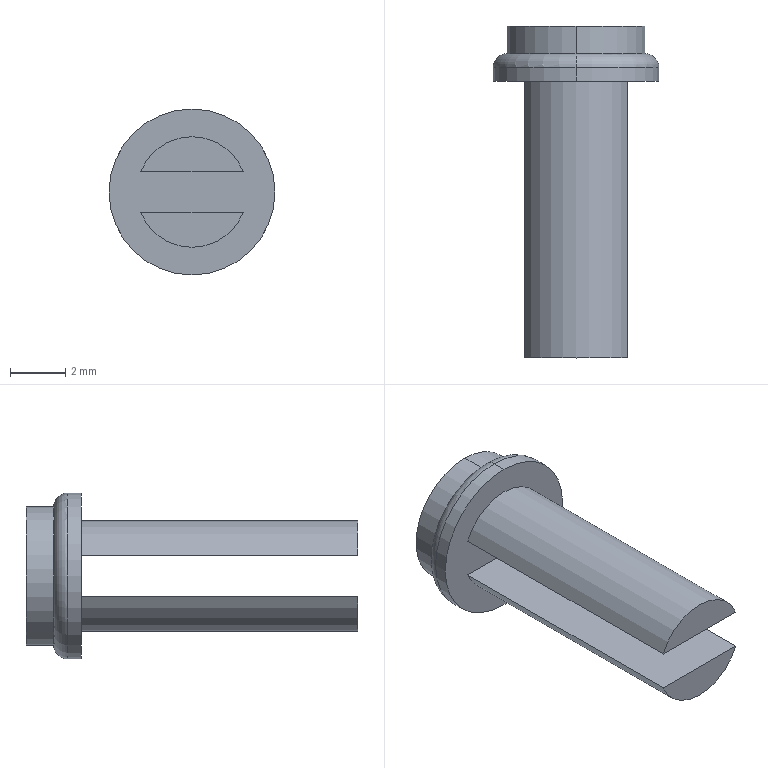Part | SolidWorks | features ICE 4, Extrusion 1, Fillet 1 | 1 solid | 28 faces | box 6 x 12 x 6 mm | volume 108.459 mm3 | plane 19 | cylinder 7 | torus 2 | commonest cylinder face diameters 4 x3 5 x2 6 x2
STEP:
#1=CARTESIAN_POINT('',(0.,10.5,-3.));
#2=VERTEX_POINT('',#1);
#3=CARTESIAN_POINT('',(0.,10.5,3.));
#4=VERTEX_POINT('',#3);
#5=CARTESIAN_POINT('',(0.,10.5,0.));
#6=DIRECTION('',(0.,-1.,0.));
#7=DIRECTION('',(0.,0.,1.));
#8=AXIS2_PLACEMENT_3D('',#5,#6,#7);
#9=CIRCLE('',#8,3.);
#10=EDGE_CURVE('',#2,#4,#9,.T.);
#11=ORIENTED_EDGE('',*,*,#10,.F.);
#12=CARTESIAN_POINT('',(0.,11.,-2.5));
#13=VERTEX_POINT('',#12);
#14=CARTESIAN_POINT('',(0.,10.5,-2.5));
#15=DIRECTION('',(1.,0.,0.));
#16=DIRECTION('',(0.,0.,-1.));
#17=AXIS2_PLACEMENT_3D('',#14,#15,#16);
#18=CIRCLE('',#17,0.5);
#19=EDGE_CURVE('',#2,#13,#18,.T.);
#20=ORIENTED_EDGE('',*,*,#19,.T.);
#21=CARTESIAN_POINT('',(0.,11.,2.5));
#22=VERTEX_POINT('',#21);
#23=CARTESIAN_POINT('',(0.,11.,0.));
#24=DIRECTION('',(0.,1.,0.));
#25=DIRECTION('',(0.,0.,1.));
#26=AXIS2_PLACEMENT_3D('',#23,#24,#25);
#27=CIRCLE('',#26,2.5);
#28=EDGE_CURVE('',#22,#13,#27,.T.);
#29=ORIENTED_EDGE('',*,*,#28,.F.);
#30=CARTESIAN_POINT('',(0.,10.5,2.5));
#31=DIRECTION('',(-1.,0.,0.));
#32=DIRECTION('',(0.,0.,1.));
#33=AXIS2_PLACEMENT_3D('',#30,#31,#32);
#34=CIRCLE('',#33,0.5);
#35=EDGE_CURVE('',#4,#22,#34,.T.);
#36=ORIENTED_EDGE('',*,*,#35,.F.);
#37=EDGE_LOOP('',(#11,#20,#29,#36));
#38=FACE_OUTER_BOUND('',#37,.T.);
#39=CARTESIAN_POINT('',(0.,10.5,0.));
#40=DIRECTION('',(0.,1.,0.));
#41=DIRECTION('',(0.,0.,1.));
#42=AXIS2_PLACEMENT_3D('',#39,#40,#41);
#43=TOROIDAL_SURFACE('',#42,2.5,0.5);
#44=ADVANCED_FACE('',(#38),#43,.T.);
#45=CARTESIAN_POINT('',(0.,12.,2.5));
#46=VERTEX_POINT('',#45);
#47=CARTESIAN_POINT('',(0.,12.,-2.5));
#48=VERTEX_POINT('',#47);
#49=CARTESIAN_POINT('',(0.,12.,0.));
#50=DIRECTION('',(0.,1.,0.));
#51=DIRECTION('',(0.,0.,1.));
#52=AXIS2_PLACEMENT_3D('',#49,#50,#51);
#53=CIRCLE('',#52,2.5);
#54=EDGE_CURVE('',#46,#48,#53,.T.);
#55=ORIENTED_EDGE('',*,*,#54,.F.);
#56=CARTESIAN_POINT('',(0.,12.,2.5));
#57=DIRECTION('',(0.,-1.,0.));
#58=VECTOR('',#57,1000.);
#59=LINE('',#56,#58);
#60=EDGE_CURVE('',#46,#22,#59,.T.);
#61=ORIENTED_EDGE('',*,*,#60,.T.);
#62=ORIENTED_EDGE('',*,*,#28,.T.);
#63=CARTESIAN_POINT('',(0.,12.,-2.5));
#64=DIRECTION('',(0.,-1.,0.));
#65=VECTOR('',#64,1000.);
#66=LINE('',#63,#65);
#67=EDGE_CURVE('',#48,#13,#66,.T.);
#68=ORIENTED_EDGE('',*,*,#67,.F.);
#69=EDGE_LOOP('',(#55,#61,#62,#68));
#70=FACE_OUTER_BOUND('',#69,.T.);
#71=CARTESIAN_POINT('',(0.,12.,0.));
#72=DIRECTION('',(0.,-1.,0.));
#73=DIRECTION('',(0.,0.,-1.));
#74=AXIS2_PLACEMENT_3D('',#71,#72,#73);
#75=CYLINDRICAL_SURFACE('',#74,2.5);
#76=ADVANCED_FACE('',(#70),#75,.T.);
#77=ORIENTED_EDGE('',*,*,#10,.T.);
#78=CARTESIAN_POINT('',(0.,10.,3.));
#79=VERTEX_POINT('',#78);
#80=CARTESIAN_POINT('',(0.,11.,3.));
#81=DIRECTION('',(0.,-1.,0.));
#82=VECTOR('',#81,1000.);
#83=LINE('',#80,#82);
#84=EDGE_CURVE('',#4,#79,#83,.T.);
#85=ORIENTED_EDGE('',*,*,#84,.T.);
#86=CARTESIAN_POINT('',(0.,10.,-3.));
#87=VERTEX_POINT('',#86);
#88=CARTESIAN_POINT('',(0.,10.,0.));
#89=DIRECTION('',(0.,1.,0.));
#90=DIRECTION('',(0.,0.,1.));
#91=AXIS2_PLACEMENT_3D('',#88,#89,#90);
#92=CIRCLE('',#91,3.);
#93=EDGE_CURVE('',#79,#87,#92,.T.);
#94=ORIENTED_EDGE('',*,*,#93,.T.);
#95=CARTESIAN_POINT('',(0.,11.,-3.));
#96=DIRECTION('',(0.,-1.,0.));
#97=VECTOR('',#96,1000.);
#98=LINE('',#95,#97);
#99=EDGE_CURVE('',#2,#87,#98,.T.);
#100=ORIENTED_EDGE('',*,*,#99,.F.);
#101=EDGE_LOOP('',(#77,#85,#94,#100));
#102=FACE_OUTER_BOUND('',#101,.T.);
#103=CARTESIAN_POINT('',(0.,11.,0.));
#104=DIRECTION('',(0.,-1.,0.));
#105=DIRECTION('',(0.,0.,-1.));
#106=AXIS2_PLACEMENT_3D('',#103,#104,#105);
#107=CYLINDRICAL_SURFACE('',#106,3.);
#108=ADVANCED_FACE('',(#102),#107,.T.);
#109=CARTESIAN_POINT('',(0.,10.,-2.));
#110=VERTEX_POINT('',#109);
#111=CARTESIAN_POINT('',(-1.854,10.,-0.75));
#112=VERTEX_POINT('',#111);
#113=CARTESIAN_POINT('',(0.,10.,0.));
#114=DIRECTION('',(0.,1.,0.));
#115=DIRECTION('',(0.,0.,1.));
#116=AXIS2_PLACEMENT_3D('',#113,#114,#115);
#117=CIRCLE('',#116,2.);
#118=EDGE_CURVE('',#110,#112,#117,.T.);
#119=ORIENTED_EDGE('',*,*,#118,.F.);
#120=CARTESIAN_POINT('',(0.,0.,-2.));
#121=VERTEX_POINT('',#120);
#122=CARTESIAN_POINT('',(0.,10.,-2.));
#123=DIRECTION('',(0.,-1.,0.));
#124=VECTOR('',#123,1000.);
#125=LINE('',#122,#124);
#126=EDGE_CURVE('',#110,#121,#125,.T.);
#127=ORIENTED_EDGE('',*,*,#126,.T.);
#128=CARTESIAN_POINT('',(-1.854,0.,-0.75));
#129=VERTEX_POINT('',#128);
#130=CARTESIAN_POINT('',(0.,0.,0.));
#131=DIRECTION('',(0.,1.,0.));
#132=DIRECTION('',(0.,0.,1.));
#133=AXIS2_PLACEMENT_3D('',#130,#131,#132);
#134=CIRCLE('',#133,2.);
#135=EDGE_CURVE('',#121,#129,#134,.T.);
#136=ORIENTED_EDGE('',*,*,#135,.T.);
#137=CARTESIAN_POINT('',(-1.854,10.,-0.75));
#138=DIRECTION('',(0.,1.,0.));
#139=VECTOR('',#138,1000.);
#140=LINE('',#137,#139);
#141=EDGE_CURVE('',#129,#112,#140,.T.);
#142=ORIENTED_EDGE('',*,*,#141,.T.);
#143=EDGE_LOOP('',(#119,#127,#136,#142));
#144=FACE_OUTER_BOUND('',#143,.T.);
#145=CARTESIAN_POINT('',(0.,10.,0.));
#146=DIRECTION('',(0.,-1.,0.));
#147=DIRECTION('',(0.,0.,-1.));
#148=AXIS2_PLACEMENT_3D('',#145,#146,#147);
#149=CYLINDRICAL_SURFACE('',#148,2.);
#150=ADVANCED_FACE('',(#144),#149,.T.);
#151=CARTESIAN_POINT('',(-1.854,10.,0.75));
#152=VERTEX_POINT('',#151);
#153=CARTESIAN_POINT('',(1.854,10.,0.75));
#154=VERTEX_POINT('',#153);
#155=CARTESIAN_POINT('',(0.,10.,0.));
#156=DIRECTION('',(0.,1.,0.));
#157=DIRECTION('',(0.,0.,1.));
#158=AXIS2_PLACEMENT_3D('',#155,#156,#157);
#159=CIRCLE('',#158,2.);
#160=EDGE_CURVE('',#152,#154,#159,.T.);
#161=ORIENTED_EDGE('',*,*,#160,.F.);
#162=CARTESIAN_POINT('',(-1.854,0.,0.75));
#163=VERTEX_POINT('',#162);
#164=CARTESIAN_POINT('',(-1.854,10.,0.75));
#165=DIRECTION('',(0.,-1.,0.));
#166=VECTOR('',#165,1000.);
#167=LINE('',#164,#166);
#168=EDGE_CURVE('',#152,#163,#167,.T.);
#169=ORIENTED_EDGE('',*,*,#168,.T.);
#170=CARTESIAN_POINT('',(1.854,0.,0.75));
#171=VERTEX_POINT('',#170);
#172=CARTESIAN_POINT('',(0.,0.,0.));
#173=DIRECTION('',(0.,1.,0.));
#174=DIRECTION('',(0.,0.,1.));
#175=AXIS2_PLACEMENT_3D('',#172,#173,#174);
#176=CIRCLE('',#175,2.);
#177=EDGE_CURVE('',#163,#171,#176,.T.);
#178=ORIENTED_EDGE('',*,*,#177,.T.);
#179=CARTESIAN_POINT('',(1.854,10.,0.75));
#180=DIRECTION('',(0.,1.,0.));
#181=VECTOR('',#180,1000.);
#182=LINE('',#179,#181);
#183=EDGE_CURVE('',#171,#154,#182,.T.);
#184=ORIENTED_EDGE('',*,*,#183,.T.);
#185=EDGE_LOOP('',(#161,#169,#178,#184));
#186=FACE_OUTER_BOUND('',#185,.T.);
#187=CARTESIAN_POINT('',(0.,10.,0.));
#188=DIRECTION('',(0.,-1.,0.));
#189=DIRECTION('',(0.,0.,-1.));
#190=AXIS2_PLACEMENT_3D('',#187,#188,#189);
#191=CYLINDRICAL_SURFACE('',#190,2.);
#192=ADVANCED_FACE('',(#186),#191,.T.);
#193=ORIENTED_EDGE('',*,*,#177,.F.);
#194=CARTESIAN_POINT('',(-5.392,0.,0.75));
#195=DIRECTION('',(-1.,0.,0.));
#196=VECTOR('',#195,1000.);
#197=LINE('',#194,#196);
#198=EDGE_CURVE('',#171,#163,#197,.T.);
#199=ORIENTED_EDGE('',*,*,#198,.F.);
#200=EDGE_LOOP('',(#193,#199));
#201=FACE_OUTER_BOUND('',#200,.T.);
#202=CARTESIAN_POINT('',(0.,0.,0.));
#203=DIRECTION('',(0.,1.,0.));
#204=DIRECTION('',(0.,0.,1.));
#205=AXIS2_PLACEMENT_3D('',#202,#203,#204);
#206=PLANE('',#205);
#207=ADVANCED_FACE('',(#201),#206,.F.);
#208=ORIENTED_EDGE('',*,*,#126,.F.);
#209=CARTESIAN_POINT('',(1.854,10.,-0.75));
#210=VERTEX_POINT('',#209);
#211=CARTESIAN_POINT('',(0.,10.,0.));
#212=DIRECTION('',(0.,1.,0.));
#213=DIRECTION('',(0.,0.,1.));
#214=AXIS2_PLACEMENT_3D('',#211,#212,#213);
#215=CIRCLE('',#214,2.);
#216=EDGE_CURVE('',#210,#110,#215,.T.);
#217=ORIENTED_EDGE('',*,*,#216,.F.);
#218=CARTESIAN_POINT('',(1.854,0.,-0.75));
#219=VERTEX_POINT('',#218);
#220=CARTESIAN_POINT('',(1.854,10.,-0.75));
#221=DIRECTION('',(0.,-1.,0.));
#222=VECTOR('',#221,1000.);
#223=LINE('',#220,#222);
#224=EDGE_CURVE('',#210,#219,#223,.T.);
#225=ORIENTED_EDGE('',*,*,#224,.T.);
#226=CARTESIAN_POINT('',(0.,0.,0.));
#227=DIRECTION('',(0.,1.,0.));
#228=DIRECTION('',(0.,0.,1.));
#229=AXIS2_PLACEMENT_3D('',#226,#227,#228);
#230=CIRCLE('',#229,2.);
#231=EDGE_CURVE('',#219,#121,#230,.T.);
#232=ORIENTED_EDGE('',*,*,#231,.T.);
#233=EDGE_LOOP('',(#208,#217,#225,#232));
#234=FACE_OUTER_BOUND('',#233,.T.);
#235=CARTESIAN_POINT('',(0.,10.,0.));
#236=DIRECTION('',(0.,-1.,0.));
#237=DIRECTION('',(0.,0.,-1.));
#238=AXIS2_PLACEMENT_3D('',#235,#236,#237);
#239=CYLINDRICAL_SURFACE('',#238,2.);
#240=ADVANCED_FACE('',(#234),#239,.T.);
#241=ORIENTED_EDGE('',*,*,#231,.F.);
#242=CARTESIAN_POINT('',(-5.392,0.,-0.75));
#243=DIRECTION('',(1.,0.,0.));
#244=VECTOR('',#243,1000.);
#245=LINE('',#242,#244);
#246=EDGE_CURVE('',#129,#219,#245,.T.);
#247=ORIENTED_EDGE('',*,*,#246,.F.);
#248=ORIENTED_EDGE('',*,*,#135,.F.);
#249=EDGE_LOOP('',(#241,#247,#248));
#250=FACE_OUTER_BOUND('',#249,.T.);
#251=CARTESIAN_POINT('',(0.,0.,0.));
#252=DIRECTION('',(0.,1.,0.));
#253=DIRECTION('',(0.,0.,1.));
#254=AXIS2_PLACEMENT_3D('',#251,#252,#253);
#255=PLANE('',#254);
#256=ADVANCED_FACE('',(#250),#255,.F.);
#257=ORIENTED_EDGE('',*,*,#84,.F.);
#258=CARTESIAN_POINT('',(0.,10.5,0.));
#259=DIRECTION('',(0.,-1.,0.));
#260=DIRECTION('',(0.,0.,1.));
#261=AXIS2_PLACEMENT_3D('',#258,#259,#260);
#262=CIRCLE('',#261,3.);
#263=EDGE_CURVE('',#4,#2,#262,.T.);
#264=ORIENTED_EDGE('',*,*,#263,.T.);
#265=ORIENTED_EDGE('',*,*,#99,.T.);
#266=CARTESIAN_POINT('',(0.,10.,0.));
#267=DIRECTION('',(0.,1.,0.));
#268=DIRECTION('',(0.,0.,1.));
#269=AXIS2_PLACEMENT_3D('',#266,#267,#268);
#270=CIRCLE('',#269,3.);
#271=EDGE_CURVE('',#87,#79,#270,.T.);
#272=ORIENTED_EDGE('',*,*,#271,.T.);
#273=EDGE_LOOP('',(#257,#264,#265,#272));
#274=FACE_OUTER_BOUND('',#273,.T.);
#275=CARTESIAN_POINT('',(0.,11.,0.));
#276=DIRECTION('',(0.,-1.,0.));
#277=DIRECTION('',(0.,0.,-1.));
#278=AXIS2_PLACEMENT_3D('',#275,#276,#277);
#279=CYLINDRICAL_SURFACE('',#278,3.);
#280=ADVANCED_FACE('',(#274),#279,.T.);
#281=CARTESIAN_POINT('',(-5.392,10.,-0.75));
#282=DIRECTION('',(1.,0.,0.));
#283=VECTOR('',#282,1000.);
#284=LINE('',#281,#283);
#285=EDGE_CURVE('',#112,#210,#284,.T.);
#286=ORIENTED_EDGE('',*,*,#285,.T.);
#287=ORIENTED_EDGE('',*,*,#216,.T.);
#288=ORIENTED_EDGE('',*,*,#118,.T.);
#289=EDGE_LOOP('',(#286,#287,#288));
#290=FACE_BOUND('',#289,.T.);
#291=ORIENTED_EDGE('',*,*,#160,.T.);
#292=CARTESIAN_POINT('',(-5.392,10.,0.75));
#293=DIRECTION('',(-1.,0.,0.));
#294=VECTOR('',#293,1000.);
#295=LINE('',#292,#294);
#296=EDGE_CURVE('',#154,#152,#295,.T.);
#297=ORIENTED_EDGE('',*,*,#296,.T.);
#298=EDGE_LOOP('',(#291,#297));
#299=FACE_BOUND('',#298,.T.);
#300=ORIENTED_EDGE('',*,*,#271,.F.);
#301=ORIENTED_EDGE('',*,*,#93,.F.);
#302=EDGE_LOOP('',(#300,#301));
#303=FACE_OUTER_BOUND('',#302,.T.);
#304=CARTESIAN_POINT('',(0.,10.,0.));
#305=DIRECTION('',(0.,1.,0.));
#306=DIRECTION('',(0.,0.,1.));
#307=AXIS2_PLACEMENT_3D('',#304,#305,#306);
#308=PLANE('',#307);
#309=ADVANCED_FACE('',(#290,#299,#303),#308,.F.);
#310=ORIENTED_EDGE('',*,*,#60,.F.);
#311=CARTESIAN_POINT('',(0.,12.,0.));
#312=DIRECTION('',(0.,1.,0.));
#313=DIRECTION('',(0.,0.,1.));
#314=AXIS2_PLACEMENT_3D('',#311,#312,#313);
#315=CIRCLE('',#314,2.5);
#316=EDGE_CURVE('',#48,#46,#315,.T.);
#317=ORIENTED_EDGE('',*,*,#316,.F.);
#318=ORIENTED_EDGE('',*,*,#67,.T.);
#319=CARTESIAN_POINT('',(0.,11.,0.));
#320=DIRECTION('',(0.,1.,0.));
#321=DIRECTION('',(0.,0.,1.));
#322=AXIS2_PLACEMENT_3D('',#319,#320,#321);
#323=CIRCLE('',#322,2.5);
#324=EDGE_CURVE('',#13,#22,#323,.T.);
#325=ORIENTED_EDGE('',*,*,#324,.T.);
#326=EDGE_LOOP('',(#310,#317,#318,#325));
#327=FACE_OUTER_BOUND('',#326,.T.);
#328=CARTESIAN_POINT('',(0.,12.,0.));
#329=DIRECTION('',(0.,-1.,0.));
#330=DIRECTION('',(0.,0.,-1.));
#331=AXIS2_PLACEMENT_3D('',#328,#329,#330);
#332=CYLINDRICAL_SURFACE('',#331,2.5);
#333=ADVANCED_FACE('',(#327),#332,.T.);
#334=CARTESIAN_POINT('',(0.25,12.,-1.984));
#335=VERTEX_POINT('',#334);
#336=CARTESIAN_POINT('',(-0.25,12.,-1.984));
#337=VERTEX_POINT('',#336);
#338=CARTESIAN_POINT('',(-0.25,12.,-1.984));
#339=DIRECTION('',(-1.,0.,0.));
#340=VECTOR('',#339,1000.);
#341=LINE('',#338,#340);
#342=EDGE_CURVE('',#335,#337,#341,.T.);
#343=ORIENTED_EDGE('',*,*,#342,.F.);
#344=CARTESIAN_POINT('',(0.25,12.,-0.25));
#345=VERTEX_POINT('',#344);
#346=CARTESIAN_POINT('',(0.25,12.,-1.984));
#347=DIRECTION('',(0.,0.,-1.));
#348=VECTOR('',#347,1000.);
#349=LINE('',#346,#348);
#350=EDGE_CURVE('',#345,#335,#349,.T.);
#351=ORIENTED_EDGE('',*,*,#350,.F.);
#352=CARTESIAN_POINT('',(1.984,12.,-0.25));
#353=VERTEX_POINT('',#352);
#354=CARTESIAN_POINT('',(1.984,12.,-0.25));
#355=DIRECTION('',(-1.,0.,0.));
#356=VECTOR('',#355,1000.);
#357=LINE('',#354,#356);
#358=EDGE_CURVE('',#353,#345,#357,.T.);
#359=ORIENTED_EDGE('',*,*,#358,.F.);
#360=CARTESIAN_POINT('',(1.984,12.,0.25));
#361=VERTEX_POINT('',#360);
#362=CARTESIAN_POINT('',(1.984,12.,-0.25));
#363=DIRECTION('',(0.,0.,-1.));
#364=VECTOR('',#363,1000.);
#365=LINE('',#362,#364);
#366=EDGE_CURVE('',#361,#353,#365,.T.);
#367=ORIENTED_EDGE('',*,*,#366,.F.);
#368=CARTESIAN_POINT('',(0.25,12.,0.25));
#369=VERTEX_POINT('',#368);
#370=CARTESIAN_POINT('',(1.984,12.,0.25));
#371=DIRECTION('',(1.,0.,0.));
#372=VECTOR('',#371,1000.);
#373=LINE('',#370,#372);
#374=EDGE_CURVE('',#369,#361,#373,.T.);
#375=ORIENTED_EDGE('',*,*,#374,.F.);
#376=CARTESIAN_POINT('',(0.25,12.,1.984));
#377=VERTEX_POINT('',#376);
#378=CARTESIAN_POINT('',(0.25,12.,0.25));
#379=DIRECTION('',(0.,0.,-1.));
#380=VECTOR('',#379,1000.);
#381=LINE('',#378,#380);
#382=EDGE_CURVE('',#377,#369,#381,.T.);
#383=ORIENTED_EDGE('',*,*,#382,.F.);
#384=CARTESIAN_POINT('',(-0.25,12.,1.984));
#385=VERTEX_POINT('',#384);
#386=CARTESIAN_POINT('',(-0.25,12.,1.984));
#387=DIRECTION('',(1.,0.,0.));
#388=VECTOR('',#387,1000.);
#389=LINE('',#386,#388);
#390=EDGE_CURVE('',#385,#377,#389,.T.);
#391=ORIENTED_EDGE('',*,*,#390,.F.);
#392=CARTESIAN_POINT('',(-0.25,12.,0.25));
#393=VERTEX_POINT('',#392);
#394=CARTESIAN_POINT('',(-0.25,12.,0.25));
#395=DIRECTION('',(0.,0.,1.));
#396=VECTOR('',#395,1000.);
#397=LINE('',#394,#396);
#398=EDGE_CURVE('',#393,#385,#397,.T.);
#399=ORIENTED_EDGE('',*,*,#398,.F.);
#400=CARTESIAN_POINT('',(-1.984,12.,0.25));
#401=VERTEX_POINT('',#400);
#402=CARTESIAN_POINT('',(-1.984,12.,0.25));
#403=DIRECTION('',(1.,0.,0.));
#404=VECTOR('',#403,1000.);
#405=LINE('',#402,#404);
#406=EDGE_CURVE('',#401,#393,#405,.T.);
#407=ORIENTED_EDGE('',*,*,#406,.F.);
#408=CARTESIAN_POINT('',(-1.984,12.,-0.25));
#409=VERTEX_POINT('',#408);
#410=CARTESIAN_POINT('',(-1.984,12.,-0.25));
#411=DIRECTION('',(0.,0.,1.));
#412=VECTOR('',#411,1000.);
#413=LINE('',#410,#412);
#414=EDGE_CURVE('',#409,#401,#413,.T.);
#415=ORIENTED_EDGE('',*,*,#414,.F.);
#416=CARTESIAN_POINT('',(-0.25,12.,-0.25));
#417=VERTEX_POINT('',#416);
#418=CARTESIAN_POINT('',(-1.984,12.,-0.25));
#419=DIRECTION('',(-1.,0.,0.));
#420=VECTOR('',#419,1000.);
#421=LINE('',#418,#420);
#422=EDGE_CURVE('',#417,#409,#421,.T.);
#423=ORIENTED_EDGE('',*,*,#422,.F.);
#424=CARTESIAN_POINT('',(-0.25,12.,-1.984));
#425=DIRECTION('',(0.,0.,1.));
#426=VECTOR('',#425,1000.);
#427=LINE('',#424,#426);
#428=EDGE_CURVE('',#337,#417,#427,.T.);
#429=ORIENTED_EDGE('',*,*,#428,.F.);
#430=EDGE_LOOP('',(#343,#351,#359,#367,#375,#383,#391,#399,#407,#415,#423,#429));
#431=FACE_BOUND('',#430,.T.);
#432=ORIENTED_EDGE('',*,*,#316,.T.);
#433=ORIENTED_EDGE('',*,*,#54,.T.);
#434=EDGE_LOOP('',(#432,#433));
#435=FACE_OUTER_BOUND('',#434,.T.);
#436=CARTESIAN_POINT('',(0.,12.,0.));
#437=DIRECTION('',(0.,1.,0.));
#438=DIRECTION('',(0.,0.,1.));
#439=AXIS2_PLACEMENT_3D('',#436,#437,#438);
#440=PLANE('',#439);
#441=ADVANCED_FACE('',(#431,#435),#440,.T.);
#442=ORIENTED_EDGE('',*,*,#342,.T.);
#443=CARTESIAN_POINT('',(-0.25,10.5,-1.984));
#444=VERTEX_POINT('',#443);
#445=CARTESIAN_POINT('',(-0.25,10.5,-1.984));
#446=DIRECTION('',(0.,1.,0.));
#447=VECTOR('',#446,1000.);
#448=LINE('',#445,#447);
#449=EDGE_CURVE('',#444,#337,#448,.T.);
#450=ORIENTED_EDGE('',*,*,#449,.F.);
#451=CARTESIAN_POINT('',(0.25,10.5,-1.984));
#452=VERTEX_POINT('',#451);
#453=CARTESIAN_POINT('',(-0.25,10.5,-1.984));
#454=DIRECTION('',(-1.,0.,0.));
#455=VECTOR('',#454,1000.);
#456=LINE('',#453,#455);
#457=EDGE_CURVE('',#452,#444,#456,.T.);
#458=ORIENTED_EDGE('',*,*,#457,.F.);
#459=CARTESIAN_POINT('',(0.25,10.5,-1.984));
#460=DIRECTION('',(0.,1.,0.));
#461=VECTOR('',#460,1000.);
#462=LINE('',#459,#461);
#463=EDGE_CURVE('',#452,#335,#462,.T.);
#464=ORIENTED_EDGE('',*,*,#463,.T.);
#465=EDGE_LOOP('',(#442,#450,#458,#464));
#466=FACE_OUTER_BOUND('',#465,.T.);
#467=CARTESIAN_POINT('',(-0.25,10.5,-1.984));
#468=DIRECTION('',(0.,0.,-1.));
#469=DIRECTION('',(-1.,0.,0.));
#470=AXIS2_PLACEMENT_3D('',#467,#468,#469);
#471=PLANE('',#470);
#472=ADVANCED_FACE('',(#466),#471,.F.);
#473=ORIENTED_EDGE('',*,*,#350,.T.);
#474=ORIENTED_EDGE('',*,*,#463,.F.);
#475=CARTESIAN_POINT('',(0.25,10.5,-0.25));
#476=VERTEX_POINT('',#475);
#477=CARTESIAN_POINT('',(0.25,10.5,-1.984));
#478=DIRECTION('',(0.,0.,-1.));
#479=VECTOR('',#478,1000.);
#480=LINE('',#477,#479);
#481=EDGE_CURVE('',#476,#452,#480,.T.);
#482=ORIENTED_EDGE('',*,*,#481,.F.);
#483=CARTESIAN_POINT('',(0.25,10.5,-0.25));
#484=DIRECTION('',(0.,1.,0.));
#485=VECTOR('',#484,1000.);
#486=LINE('',#483,#485);
#487=EDGE_CURVE('',#476,#345,#486,.T.);
#488=ORIENTED_EDGE('',*,*,#487,.T.);
#489=EDGE_LOOP('',(#473,#474,#482,#488));
#490=FACE_OUTER_BOUND('',#489,.T.);
#491=CARTESIAN_POINT('',(0.25,10.5,-1.984));
#492=DIRECTION('',(1.,0.,0.));
#493=DIRECTION('',(0.,0.,-1.));
#494=AXIS2_PLACEMENT_3D('',#491,#492,#493);
#495=PLANE('',#494);
#496=ADVANCED_FACE('',(#490),#495,.F.);
#497=ORIENTED_EDGE('',*,*,#358,.T.);
#498=ORIENTED_EDGE('',*,*,#487,.F.);
#499=CARTESIAN_POINT('',(1.984,10.5,-0.25));
#500=VERTEX_POINT('',#499);
#501=CARTESIAN_POINT('',(1.984,10.5,-0.25));
#502=DIRECTION('',(-1.,0.,0.));
#503=VECTOR('',#502,1000.);
#504=LINE('',#501,#503);
#505=EDGE_CURVE('',#500,#476,#504,.T.);
#506=ORIENTED_EDGE('',*,*,#505,.F.);
#507=CARTESIAN_POINT('',(1.984,10.5,-0.25));
#508=DIRECTION('',(0.,1.,0.));
#509=VECTOR('',#508,1000.);
#510=LINE('',#507,#509);
#511=EDGE_CURVE('',#500,#353,#510,.T.);
#512=ORIENTED_EDGE('',*,*,#511,.T.);
#513=EDGE_LOOP('',(#497,#498,#506,#512));
#514=FACE_OUTER_BOUND('',#513,.T.);
#515=CARTESIAN_POINT('',(1.984,10.5,-0.25));
#516=DIRECTION('',(0.,0.,-1.));
#517=DIRECTION('',(-1.,0.,0.));
#518=AXIS2_PLACEMENT_3D('',#515,#516,#517);
#519=PLANE('',#518);
#520=ADVANCED_FACE('',(#514),#519,.F.);
#521=ORIENTED_EDGE('',*,*,#366,.T.);
#522=ORIENTED_EDGE('',*,*,#511,.F.);
#523=CARTESIAN_POINT('',(1.984,10.5,0.25));
#524=VERTEX_POINT('',#523);
#525=CARTESIAN_POINT('',(1.984,10.5,-0.25));
#526=DIRECTION('',(0.,0.,-1.));
#527=VECTOR('',#526,1000.);
#528=LINE('',#525,#527);
#529=EDGE_CURVE('',#524,#500,#528,.T.);
#530=ORIENTED_EDGE('',*,*,#529,.F.);
#531=CARTESIAN_POINT('',(1.984,10.5,0.25));
#532=DIRECTION('',(0.,1.,0.));
#533=VECTOR('',#532,1000.);
#534=LINE('',#531,#533);
#535=EDGE_CURVE('',#524,#361,#534,.T.);
#536=ORIENTED_EDGE('',*,*,#535,.T.);
#537=EDGE_LOOP('',(#521,#522,#530,#536));
#538=FACE_OUTER_BOUND('',#537,.T.);
#539=CARTESIAN_POINT('',(1.984,10.5,-0.25));
#540=DIRECTION('',(1.,0.,0.));
#541=DIRECTION('',(0.,0.,-1.));
#542=AXIS2_PLACEMENT_3D('',#539,#540,#541);
#543=PLANE('',#542);
#544=ADVANCED_FACE('',(#538),#543,.F.);
#545=ORIENTED_EDGE('',*,*,#374,.T.);
#546=ORIENTED_EDGE('',*,*,#535,.F.);
#547=CARTESIAN_POINT('',(0.25,10.5,0.25));
#548=VERTEX_POINT('',#547);
#549=CARTESIAN_POINT('',(1.984,10.5,0.25));
#550=DIRECTION('',(1.,0.,0.));
#551=VECTOR('',#550,1000.);
#552=LINE('',#549,#551);
#553=EDGE_CURVE('',#548,#524,#552,.T.);
#554=ORIENTED_EDGE('',*,*,#553,.F.);
#555=CARTESIAN_POINT('',(0.25,10.5,0.25));
#556=DIRECTION('',(0.,1.,0.));
#557=VECTOR('',#556,1000.);
#558=LINE('',#555,#557);
#559=EDGE_CURVE('',#548,#369,#558,.T.);
#560=ORIENTED_EDGE('',*,*,#559,.T.);
#561=EDGE_LOOP('',(#545,#546,#554,#560));
#562=FACE_OUTER_BOUND('',#561,.T.);
#563=CARTESIAN_POINT('',(1.984,10.5,0.25));
#564=DIRECTION('',(0.,0.,1.));
#565=DIRECTION('',(1.,0.,0.));
#566=AXIS2_PLACEMENT_3D('',#563,#564,#565);
#567=PLANE('',#566);
#568=ADVANCED_FACE('',(#562),#567,.F.);
#569=ORIENTED_EDGE('',*,*,#382,.T.);
#570=ORIENTED_EDGE('',*,*,#559,.F.);
#571=CARTESIAN_POINT('',(0.25,10.5,1.984));
#572=VERTEX_POINT('',#571);
#573=CARTESIAN_POINT('',(0.25,10.5,0.25));
#574=DIRECTION('',(0.,0.,-1.));
#575=VECTOR('',#574,1000.);
#576=LINE('',#573,#575);
#577=EDGE_CURVE('',#572,#548,#576,.T.);
#578=ORIENTED_EDGE('',*,*,#577,.F.);
#579=CARTESIAN_POINT('',(0.25,10.5,1.984));
#580=DIRECTION('',(0.,1.,0.));
#581=VECTOR('',#580,1000.);
#582=LINE('',#579,#581);
#583=EDGE_CURVE('',#572,#377,#582,.T.);
#584=ORIENTED_EDGE('',*,*,#583,.T.);
#585=EDGE_LOOP('',(#569,#570,#578,#584));
#586=FACE_OUTER_BOUND('',#585,.T.);
#587=CARTESIAN_POINT('',(0.25,10.5,0.25));
#588=DIRECTION('',(1.,0.,0.));
#589=DIRECTION('',(0.,0.,-1.));
#590=AXIS2_PLACEMENT_3D('',#587,#588,#589);
#591=PLANE('',#590);
#592=ADVANCED_FACE('',(#586),#591,.F.);
#593=ORIENTED_EDGE('',*,*,#390,.T.);
#594=ORIENTED_EDGE('',*,*,#583,.F.);
#595=CARTESIAN_POINT('',(-0.25,10.5,1.984));
#596=VERTEX_POINT('',#595);
#597=CARTESIAN_POINT('',(-0.25,10.5,1.984));
#598=DIRECTION('',(1.,0.,0.));
#599=VECTOR('',#598,1000.);
#600=LINE('',#597,#599);
#601=EDGE_CURVE('',#596,#572,#600,.T.);
#602=ORIENTED_EDGE('',*,*,#601,.F.);
#603=CARTESIAN_POINT('',(-0.25,10.5,1.984));
#604=DIRECTION('',(0.,1.,0.));
#605=VECTOR('',#604,1000.);
#606=LINE('',#603,#605);
#607=EDGE_CURVE('',#596,#385,#606,.T.);
#608=ORIENTED_EDGE('',*,*,#607,.T.);
#609=EDGE_LOOP('',(#593,#594,#602,#608));
#610=FACE_OUTER_BOUND('',#609,.T.);
#611=CARTESIAN_POINT('',(-0.25,10.5,1.984));
#612=DIRECTION('',(0.,0.,1.));
#613=DIRECTION('',(1.,0.,0.));
#614=AXIS2_PLACEMENT_3D('',#611,#612,#613);
#615=PLANE('',#614);
#616=ADVANCED_FACE('',(#610),#615,.F.);
#617=ORIENTED_EDGE('',*,*,#398,.T.);
#618=ORIENTED_EDGE('',*,*,#607,.F.);
#619=CARTESIAN_POINT('',(-0.25,10.5,0.25));
#620=VERTEX_POINT('',#619);
#621=CARTESIAN_POINT('',(-0.25,10.5,0.25));
#622=DIRECTION('',(0.,0.,1.));
#623=VECTOR('',#622,1000.);
#624=LINE('',#621,#623);
#625=EDGE_CURVE('',#620,#596,#624,.T.);
#626=ORIENTED_EDGE('',*,*,#625,.F.);
#627=CARTESIAN_POINT('',(-0.25,10.5,0.25));
#628=DIRECTION('',(0.,1.,0.));
#629=VECTOR('',#628,1000.);
#630=LINE('',#627,#629);
#631=EDGE_CURVE('',#620,#393,#630,.T.);
#632=ORIENTED_EDGE('',*,*,#631,.T.);
#633=EDGE_LOOP('',(#617,#618,#626,#632));
#634=FACE_OUTER_BOUND('',#633,.T.);
#635=CARTESIAN_POINT('',(-0.25,10.5,0.25));
#636=DIRECTION('',(-1.,0.,0.));
#637=DIRECTION('',(0.,0.,1.));
#638=AXIS2_PLACEMENT_3D('',#635,#636,#637);
#639=PLANE('',#638);
#640=ADVANCED_FACE('',(#634),#639,.F.);
#641=ORIENTED_EDGE('',*,*,#406,.T.);
#642=ORIENTED_EDGE('',*,*,#631,.F.);
#643=CARTESIAN_POINT('',(-1.984,10.5,0.25));
#644=VERTEX_POINT('',#643);
#645=CARTESIAN_POINT('',(-1.984,10.5,0.25));
#646=DIRECTION('',(1.,0.,0.));
#647=VECTOR('',#646,1000.);
#648=LINE('',#645,#647);
#649=EDGE_CURVE('',#644,#620,#648,.T.);
#650=ORIENTED_EDGE('',*,*,#649,.F.);
#651=CARTESIAN_POINT('',(-1.984,10.5,0.25));
#652=DIRECTION('',(0.,1.,0.));
#653=VECTOR('',#652,1000.);
#654=LINE('',#651,#653);
#655=EDGE_CURVE('',#644,#401,#654,.T.);
#656=ORIENTED_EDGE('',*,*,#655,.T.);
#657=EDGE_LOOP('',(#641,#642,#650,#656));
#658=FACE_OUTER_BOUND('',#657,.T.);
#659=CARTESIAN_POINT('',(-1.984,10.5,0.25));
#660=DIRECTION('',(0.,0.,1.));
#661=DIRECTION('',(1.,0.,0.));
#662=AXIS2_PLACEMENT_3D('',#659,#660,#661);
#663=PLANE('',#662);
#664=ADVANCED_FACE('',(#658),#663,.F.);
#665=ORIENTED_EDGE('',*,*,#414,.T.);
#666=ORIENTED_EDGE('',*,*,#655,.F.);
#667=CARTESIAN_POINT('',(-1.984,10.5,-0.25));
#668=VERTEX_POINT('',#667);
#669=CARTESIAN_POINT('',(-1.984,10.5,-0.25));
#670=DIRECTION('',(0.,0.,1.));
#671=VECTOR('',#670,1000.);
#672=LINE('',#669,#671);
#673=EDGE_CURVE('',#668,#644,#672,.T.);
#674=ORIENTED_EDGE('',*,*,#673,.F.);
#675=CARTESIAN_POINT('',(-1.984,10.5,-0.25));
#676=DIRECTION('',(0.,1.,0.));
#677=VECTOR('',#676,1000.);
#678=LINE('',#675,#677);
#679=EDGE_CURVE('',#668,#409,#678,.T.);
#680=ORIENTED_EDGE('',*,*,#679,.T.);
#681=EDGE_LOOP('',(#665,#666,#674,#680));
#682=FACE_OUTER_BOUND('',#681,.T.);
#683=CARTESIAN_POINT('',(-1.984,10.5,-0.25));
#684=DIRECTION('',(-1.,0.,0.));
#685=DIRECTION('',(0.,0.,1.));
#686=AXIS2_PLACEMENT_3D('',#683,#684,#685);
#687=PLANE('',#686);
#688=ADVANCED_FACE('',(#682),#687,.F.);
#689=ORIENTED_EDGE('',*,*,#422,.T.);
#690=ORIENTED_EDGE('',*,*,#679,.F.);
#691=CARTESIAN_POINT('',(-0.25,10.5,-0.25));
#692=VERTEX_POINT('',#691);
#693=CARTESIAN_POINT('',(-1.984,10.5,-0.25));
#694=DIRECTION('',(-1.,0.,0.));
#695=VECTOR('',#694,1000.);
#696=LINE('',#693,#695);
#697=EDGE_CURVE('',#692,#668,#696,.T.);
#698=ORIENTED_EDGE('',*,*,#697,.F.);
#699=CARTESIAN_POINT('',(-0.25,10.5,-0.25));
#700=DIRECTION('',(0.,1.,0.));
#701=VECTOR('',#700,1000.);
#702=LINE('',#699,#701);
#703=EDGE_CURVE('',#692,#417,#702,.T.);
#704=ORIENTED_EDGE('',*,*,#703,.T.);
#705=EDGE_LOOP('',(#689,#690,#698,#704));
#706=FACE_OUTER_BOUND('',#705,.T.);
#707=CARTESIAN_POINT('',(-1.984,10.5,-0.25));
#708=DIRECTION('',(0.,0.,-1.));
#709=DIRECTION('',(-1.,0.,0.));
#710=AXIS2_PLACEMENT_3D('',#707,#708,#709);
#711=PLANE('',#710);
#712=ADVANCED_FACE('',(#706),#711,.F.);
#713=ORIENTED_EDGE('',*,*,#428,.T.);
#714=ORIENTED_EDGE('',*,*,#703,.F.);
#715=CARTESIAN_POINT('',(-0.25,10.5,-1.984));
#716=DIRECTION('',(0.,0.,1.));
#717=VECTOR('',#716,1000.);
#718=LINE('',#715,#717);
#719=EDGE_CURVE('',#444,#692,#718,.T.);
#720=ORIENTED_EDGE('',*,*,#719,.F.);
#721=ORIENTED_EDGE('',*,*,#449,.T.);
#722=EDGE_LOOP('',(#713,#714,#720,#721));
#723=FACE_OUTER_BOUND('',#722,.T.);
#724=CARTESIAN_POINT('',(-0.25,10.5,-1.984));
#725=DIRECTION('',(-1.,0.,0.));
#726=DIRECTION('',(0.,0.,1.));
#727=AXIS2_PLACEMENT_3D('',#724,#725,#726);
#728=PLANE('',#727);
#729=ADVANCED_FACE('',(#723),#728,.F.);
#730=ORIENTED_EDGE('',*,*,#457,.T.);
#731=ORIENTED_EDGE('',*,*,#719,.T.);
#732=ORIENTED_EDGE('',*,*,#697,.T.);
#733=ORIENTED_EDGE('',*,*,#673,.T.);
#734=ORIENTED_EDGE('',*,*,#649,.T.);
#735=ORIENTED_EDGE('',*,*,#625,.T.);
#736=ORIENTED_EDGE('',*,*,#601,.T.);
#737=ORIENTED_EDGE('',*,*,#577,.T.);
#738=ORIENTED_EDGE('',*,*,#553,.T.);
#739=ORIENTED_EDGE('',*,*,#529,.T.);
#740=ORIENTED_EDGE('',*,*,#505,.T.);
#741=ORIENTED_EDGE('',*,*,#481,.T.);
#742=EDGE_LOOP('',(#730,#731,#732,#733,#734,#735,#736,#737,#738,#739,#740,#741));
#743=FACE_OUTER_BOUND('',#742,.T.);
#744=CARTESIAN_POINT('',(0.,10.5,0.));
#745=DIRECTION('',(0.,-1.,0.));
#746=DIRECTION('',(0.,0.,-1.));
#747=AXIS2_PLACEMENT_3D('',#744,#745,#746);
#748=PLANE('',#747);
#749=ADVANCED_FACE('',(#743),#748,.F.);
#750=ORIENTED_EDGE('',*,*,#19,.F.);
#751=ORIENTED_EDGE('',*,*,#263,.F.);
#752=ORIENTED_EDGE('',*,*,#35,.T.);
#753=ORIENTED_EDGE('',*,*,#324,.F.);
#754=EDGE_LOOP('',(#750,#751,#752,#753));
#755=FACE_OUTER_BOUND('',#754,.T.);
#756=CARTESIAN_POINT('',(0.,10.5,0.));
#757=DIRECTION('',(0.,1.,0.));
#758=DIRECTION('',(0.,0.,1.));
#759=AXIS2_PLACEMENT_3D('',#756,#757,#758);
#760=TOROIDAL_SURFACE('',#759,2.5,0.5);
#761=ADVANCED_FACE('',(#755),#760,.T.);
#762=ORIENTED_EDGE('',*,*,#296,.F.);
#763=ORIENTED_EDGE('',*,*,#183,.F.);
#764=ORIENTED_EDGE('',*,*,#198,.T.);
#765=ORIENTED_EDGE('',*,*,#168,.F.);
#766=EDGE_LOOP('',(#762,#763,#764,#765));
#767=FACE_OUTER_BOUND('',#766,.T.);
#768=CARTESIAN_POINT('',(-5.392,20.888,0.75));
#769=DIRECTION('',(0.,0.,1.));
#770=DIRECTION('',(1.,0.,0.));
#771=AXIS2_PLACEMENT_3D('',#768,#769,#770);
#772=PLANE('',#771);
#773=ADVANCED_FACE('',(#767),#772,.F.);
#774=ORIENTED_EDGE('',*,*,#285,.F.);
#775=ORIENTED_EDGE('',*,*,#141,.F.);
#776=ORIENTED_EDGE('',*,*,#246,.T.);
#777=ORIENTED_EDGE('',*,*,#224,.F.);
#778=EDGE_LOOP('',(#774,#775,#776,#777));
#779=FACE_OUTER_BOUND('',#778,.T.);
#780=CARTESIAN_POINT('',(-5.392,20.888,-0.75));
#781=DIRECTION('',(0.,0.,-1.));
#782=DIRECTION('',(-1.,0.,0.));
#783=AXIS2_PLACEMENT_3D('',#780,#781,#782);
#784=PLANE('',#783);
#785=ADVANCED_FACE('',(#779),#784,.F.);
#786=CLOSED_SHELL('',(#44,#76,#108,#150,#192,#207,#240,#256,#280,#309,#333,#441,#472,#496,#520,#544,#568,#592,#616,#640,#664,#688,#712,#729,#749,#761,#773,#785));
#787=MANIFOLD_SOLID_BREP('',#786);
#788=CARTESIAN_POINT('',(0.,0.,0.));
#789=DIRECTION('',(0.,0.,1.));
#790=DIRECTION('',(1.,0.,0.));
#791=AXIS2_PLACEMENT_3D('',#788,#789,#790);
#792=(LENGTH_UNIT()NAMED_UNIT(*)SI_UNIT(.MILLI.,.METRE.));
#793=UNCERTAINTY_MEASURE_WITH_UNIT(LENGTH_MEASURE(0.00001),#792,'','');
#794=(NAMED_UNIT(*)PLANE_ANGLE_UNIT()SI_UNIT($,.RADIAN.));
#795=(NAMED_UNIT(*)SI_UNIT($,.STERADIAN.)SOLID_ANGLE_UNIT());
#796=(GEOMETRIC_REPRESENTATION_CONTEXT(3)GLOBAL_UNCERTAINTY_ASSIGNED_CONTEXT((#793))GLOBAL_UNIT_ASSIGNED_CONTEXT((#792,#794,#795))REPRESENTATION_CONTEXT('',''));
#797=ADVANCED_BREP_SHAPE_REPRESENTATION('',(#787,#791),#796);